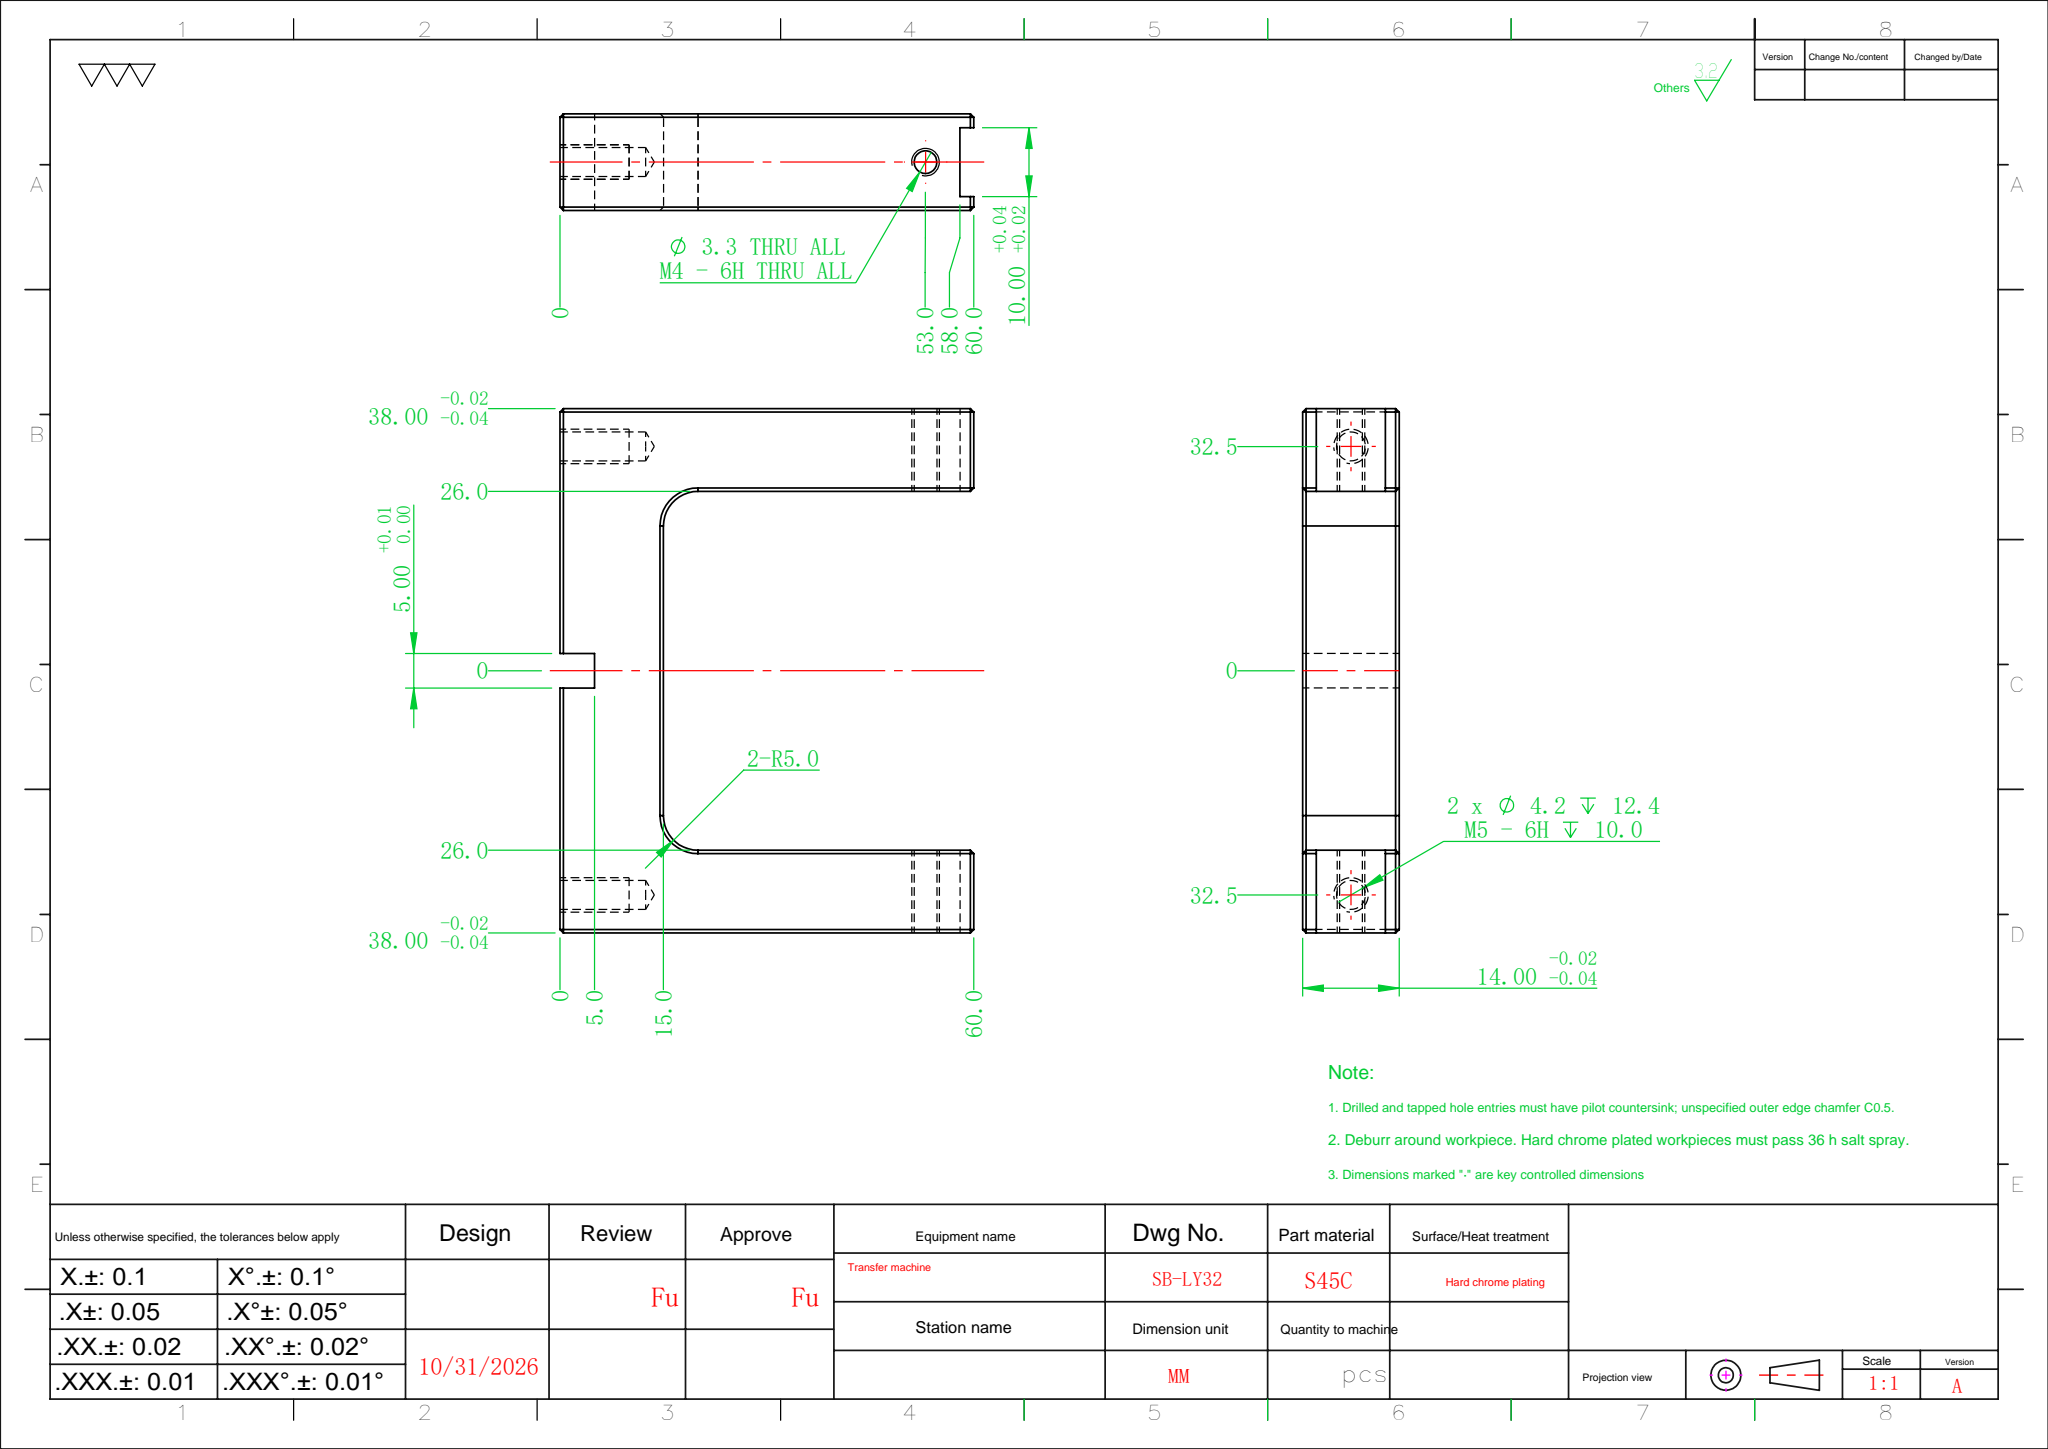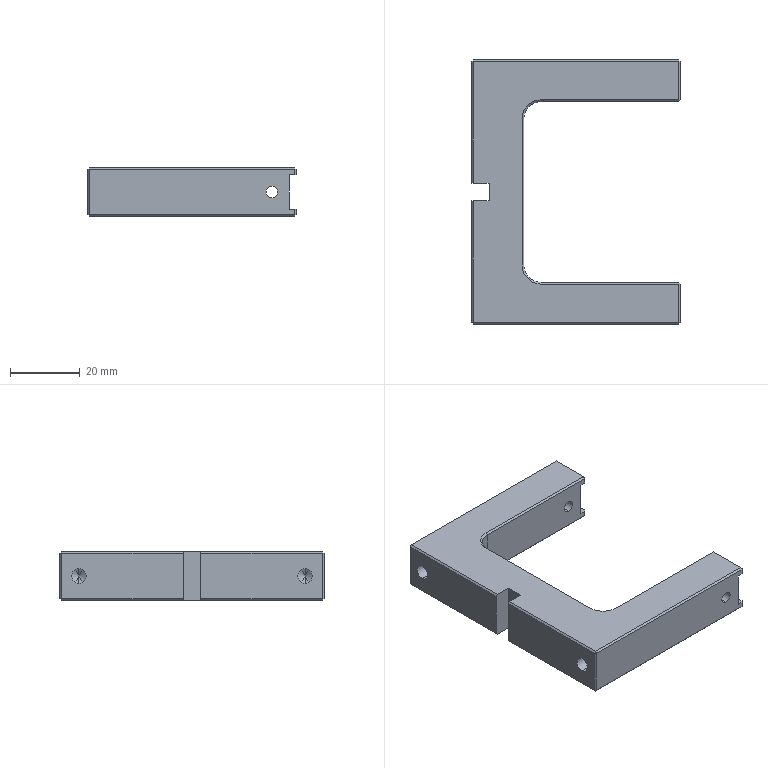Part | SolidWorks | features Cut 2, HoleWzd 2, Chamfer 1, Extrusion 1, Fillet 1, ICE 1 | 1 solid | 80 faces | box 60 x 76 x 14 mm | volume 29747 mm3 | plane 62 | cylinder 10 | cone 8 | commonest cylinder face diameters 3.3 x4 4.2 x4 10 x2